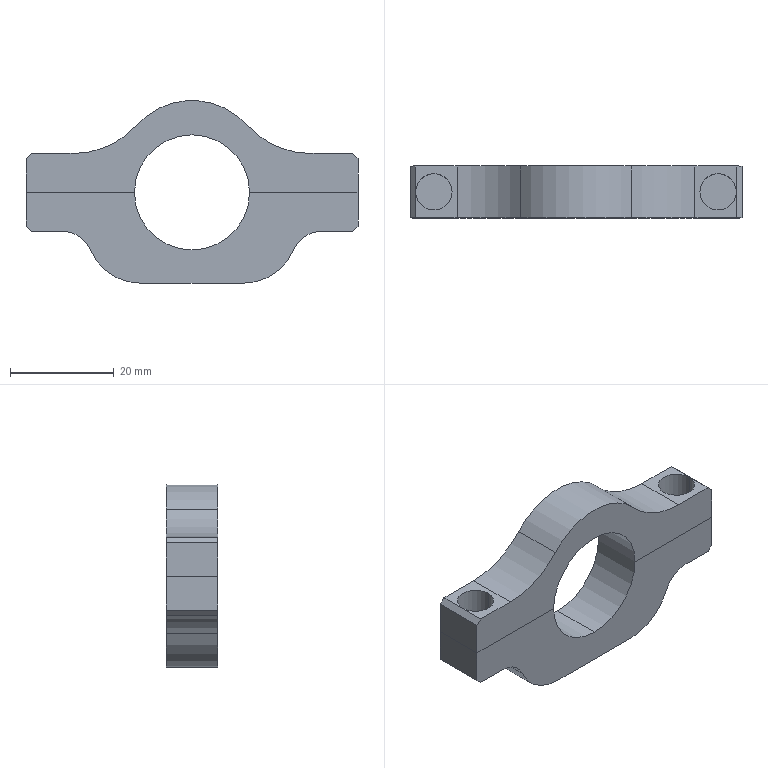Part | SolidWorks | features ICE 2, Chamfer 1, Extrusion 1, PLine 1 | 1 solid | 32 faces | box 64 x 10 x 35.214 mm | volume 11091 mm3 | plane 19 | cylinder 13 | commonest cylinder face diameters 7 x4 11.692 x2 21.037 x2 22.2 x2 33.122 x2 28.569 x1
STEP:
#1=CARTESIAN_POINT('',(0.,0.,-6.346));
#2=VERTEX_POINT('',#1);
#3=CARTESIAN_POINT('',(-11.1,0.,4.754));
#4=VERTEX_POINT('',#3);
#5=CARTESIAN_POINT('',(0.,0.,4.754));
#6=DIRECTION('',(0.,1.,0.));
#7=DIRECTION('',(0.,0.,1.));
#8=AXIS2_PLACEMENT_3D('',#5,#6,#7);
#9=CIRCLE('',#8,11.1);
#10=EDGE_CURVE('',#2,#4,#9,.T.);
#11=ORIENTED_EDGE('',*,*,#10,.F.);
#12=CARTESIAN_POINT('',(0.,10.,-6.346));
#13=VERTEX_POINT('',#12);
#14=CARTESIAN_POINT('',(0.,-10.,-6.346));
#15=DIRECTION('',(0.,1.,0.));
#16=VECTOR('',#15,1000.);
#17=LINE('',#14,#16);
#18=EDGE_CURVE('',#2,#13,#17,.T.);
#19=ORIENTED_EDGE('',*,*,#18,.T.);
#20=CARTESIAN_POINT('',(-11.1,10.,4.754));
#21=VERTEX_POINT('',#20);
#22=CARTESIAN_POINT('',(0.,10.,4.754));
#23=DIRECTION('',(0.,1.,0.));
#24=DIRECTION('',(0.,0.,1.));
#25=AXIS2_PLACEMENT_3D('',#22,#23,#24);
#26=CIRCLE('',#25,11.1);
#27=EDGE_CURVE('',#13,#21,#26,.T.);
#28=ORIENTED_EDGE('',*,*,#27,.T.);
#29=CARTESIAN_POINT('',(0.,10.,15.854));
#30=VERTEX_POINT('',#29);
#31=CARTESIAN_POINT('',(0.,10.,4.754));
#32=DIRECTION('',(0.,1.,0.));
#33=DIRECTION('',(0.,0.,1.));
#34=AXIS2_PLACEMENT_3D('',#31,#32,#33);
#35=CIRCLE('',#34,11.1);
#36=EDGE_CURVE('',#21,#30,#35,.T.);
#37=ORIENTED_EDGE('',*,*,#36,.T.);
#38=CARTESIAN_POINT('',(0.,0.,15.854));
#39=VERTEX_POINT('',#38);
#40=CARTESIAN_POINT('',(0.,-10.,15.854));
#41=DIRECTION('',(0.,1.,0.));
#42=VECTOR('',#41,1000.);
#43=LINE('',#40,#42);
#44=EDGE_CURVE('',#39,#30,#43,.T.);
#45=ORIENTED_EDGE('',*,*,#44,.F.);
#46=CARTESIAN_POINT('',(0.,0.,4.754));
#47=DIRECTION('',(0.,1.,0.));
#48=DIRECTION('',(0.,0.,1.));
#49=AXIS2_PLACEMENT_3D('',#46,#47,#48);
#50=CIRCLE('',#49,11.1);
#51=EDGE_CURVE('',#4,#39,#50,.T.);
#52=ORIENTED_EDGE('',*,*,#51,.F.);
#53=EDGE_LOOP('',(#11,#19,#28,#37,#45,#52));
#54=FACE_OUTER_BOUND('',#53,.T.);
#55=CARTESIAN_POINT('',(0.,-10.,4.754));
#56=DIRECTION('',(0.,1.,0.));
#57=DIRECTION('',(0.,0.,1.));
#58=AXIS2_PLACEMENT_3D('',#55,#56,#57);
#59=CYLINDRICAL_SURFACE('',#58,11.1);
#60=ADVANCED_FACE('',(#54),#59,.F.);
#61=CARTESIAN_POINT('',(-30.901,5.,12.254));
#62=VERTEX_POINT('',#61);
#63=CARTESIAN_POINT('',(-23.901,5.,12.254));
#64=VERTEX_POINT('',#63);
#65=CARTESIAN_POINT('',(-27.401,5.,12.254));
#66=DIRECTION('',(0.,0.,1.));
#67=DIRECTION('',(-1.,0.,0.));
#68=AXIS2_PLACEMENT_3D('',#65,#66,#67);
#69=CIRCLE('',#68,3.5);
#70=EDGE_CURVE('',#62,#64,#69,.T.);
#71=ORIENTED_EDGE('',*,*,#70,.T.);
#72=CARTESIAN_POINT('',(-23.901,5.,4.754));
#73=VERTEX_POINT('',#72);
#74=CARTESIAN_POINT('',(-23.901,5.,24.754));
#75=DIRECTION('',(0.,0.,-1.));
#76=VECTOR('',#75,1000.);
#77=LINE('',#74,#76);
#78=EDGE_CURVE('',#64,#73,#77,.T.);
#79=ORIENTED_EDGE('',*,*,#78,.T.);
#80=CARTESIAN_POINT('',(-30.901,5.,4.754));
#81=VERTEX_POINT('',#80);
#82=CARTESIAN_POINT('',(-27.401,5.,4.754));
#83=DIRECTION('',(0.,0.,1.));
#84=DIRECTION('',(-1.,0.,0.));
#85=AXIS2_PLACEMENT_3D('',#82,#83,#84);
#86=CIRCLE('',#85,3.5);
#87=EDGE_CURVE('',#81,#73,#86,.T.);
#88=ORIENTED_EDGE('',*,*,#87,.F.);
#89=CARTESIAN_POINT('',(-30.901,5.,24.754));
#90=DIRECTION('',(0.,0.,-1.));
#91=VECTOR('',#90,1000.);
#92=LINE('',#89,#91);
#93=EDGE_CURVE('',#62,#81,#92,.T.);
#94=ORIENTED_EDGE('',*,*,#93,.F.);
#95=EDGE_LOOP('',(#71,#79,#88,#94));
#96=FACE_OUTER_BOUND('',#95,.T.);
#97=CARTESIAN_POINT('',(-27.401,5.,24.754));
#98=DIRECTION('',(0.,0.,-1.));
#99=DIRECTION('',(-1.,0.,0.));
#100=AXIS2_PLACEMENT_3D('',#97,#98,#99);
#101=CYLINDRICAL_SURFACE('',#100,3.5);
#102=ADVANCED_FACE('',(#96),#101,.F.);
#103=CARTESIAN_POINT('',(30.901,5.,12.254));
#104=VERTEX_POINT('',#103);
#105=CARTESIAN_POINT('',(23.901,5.,12.254));
#106=VERTEX_POINT('',#105);
#107=CARTESIAN_POINT('',(27.401,5.,12.254));
#108=DIRECTION('',(0.,0.,-1.));
#109=DIRECTION('',(1.,0.,0.));
#110=AXIS2_PLACEMENT_3D('',#107,#108,#109);
#111=CIRCLE('',#110,3.5);
#112=EDGE_CURVE('',#104,#106,#111,.T.);
#113=ORIENTED_EDGE('',*,*,#112,.F.);
#114=CARTESIAN_POINT('',(30.901,5.,4.754));
#115=VERTEX_POINT('',#114);
#116=CARTESIAN_POINT('',(30.901,5.,24.754));
#117=DIRECTION('',(0.,0.,-1.));
#118=VECTOR('',#117,1000.);
#119=LINE('',#116,#118);
#120=EDGE_CURVE('',#104,#115,#119,.T.);
#121=ORIENTED_EDGE('',*,*,#120,.T.);
#122=CARTESIAN_POINT('',(23.901,5.,4.754));
#123=VERTEX_POINT('',#122);
#124=CARTESIAN_POINT('',(27.401,5.,4.754));
#125=DIRECTION('',(0.,0.,1.));
#126=DIRECTION('',(1.,0.,0.));
#127=AXIS2_PLACEMENT_3D('',#124,#125,#126);
#128=CIRCLE('',#127,3.5);
#129=EDGE_CURVE('',#123,#115,#128,.T.);
#130=ORIENTED_EDGE('',*,*,#129,.F.);
#131=CARTESIAN_POINT('',(23.901,5.,24.754));
#132=DIRECTION('',(0.,0.,-1.));
#133=VECTOR('',#132,1000.);
#134=LINE('',#131,#133);
#135=EDGE_CURVE('',#106,#123,#134,.T.);
#136=ORIENTED_EDGE('',*,*,#135,.F.);
#137=EDGE_LOOP('',(#113,#121,#130,#136));
#138=FACE_OUTER_BOUND('',#137,.T.);
#139=CARTESIAN_POINT('',(27.401,5.,24.754));
#140=DIRECTION('',(0.,0.,-1.));
#141=DIRECTION('',(-1.,0.,0.));
#142=AXIS2_PLACEMENT_3D('',#139,#140,#141);
#143=CYLINDRICAL_SURFACE('',#142,3.5);
#144=ADVANCED_FACE('',(#138),#143,.F.);
#145=CARTESIAN_POINT('',(-32.,0.,4.754));
#146=VERTEX_POINT('',#145);
#147=CARTESIAN_POINT('',(-32.,0.,11.254));
#148=VERTEX_POINT('',#147);
#149=CARTESIAN_POINT('',(-32.,0.,0.));
#150=DIRECTION('',(0.,0.,1.));
#151=VECTOR('',#150,1000.);
#152=LINE('',#149,#151);
#153=EDGE_CURVE('',#146,#148,#152,.T.);
#154=ORIENTED_EDGE('',*,*,#153,.T.);
#155=CARTESIAN_POINT('',(-32.,10.,11.254));
#156=VERTEX_POINT('',#155);
#157=CARTESIAN_POINT('',(-32.,10.,11.254));
#158=DIRECTION('',(0.,1.,0.));
#159=VECTOR('',#158,1000.);
#160=LINE('',#157,#159);
#161=EDGE_CURVE('',#148,#156,#160,.T.);
#162=ORIENTED_EDGE('',*,*,#161,.T.);
#163=CARTESIAN_POINT('',(-32.,10.,4.754));
#164=VERTEX_POINT('',#163);
#165=CARTESIAN_POINT('',(-32.,10.,0.));
#166=DIRECTION('',(0.,0.,1.));
#167=VECTOR('',#166,1000.);
#168=LINE('',#165,#167);
#169=EDGE_CURVE('',#164,#156,#168,.T.);
#170=ORIENTED_EDGE('',*,*,#169,.F.);
#171=CARTESIAN_POINT('',(-32.,10.,4.754));
#172=DIRECTION('',(0.,1.,0.));
#173=VECTOR('',#172,1000.);
#174=LINE('',#171,#173);
#175=EDGE_CURVE('',#146,#164,#174,.T.);
#176=ORIENTED_EDGE('',*,*,#175,.F.);
#177=EDGE_LOOP('',(#154,#162,#170,#176));
#178=FACE_OUTER_BOUND('',#177,.T.);
#179=CARTESIAN_POINT('',(-32.,10.,0.));
#180=DIRECTION('',(1.,0.,0.));
#181=DIRECTION('',(0.,0.,-1.));
#182=AXIS2_PLACEMENT_3D('',#179,#180,#181);
#183=PLANE('',#182);
#184=ADVANCED_FACE('',(#178),#183,.F.);
#185=CARTESIAN_POINT('',(32.,10.,4.754));
#186=VERTEX_POINT('',#185);
#187=CARTESIAN_POINT('',(32.,10.,11.254));
#188=VERTEX_POINT('',#187);
#189=CARTESIAN_POINT('',(32.,10.,0.));
#190=DIRECTION('',(0.,0.,1.));
#191=VECTOR('',#190,1000.);
#192=LINE('',#189,#191);
#193=EDGE_CURVE('',#186,#188,#192,.T.);
#194=ORIENTED_EDGE('',*,*,#193,.T.);
#195=CARTESIAN_POINT('',(32.,0.,11.254));
#196=VERTEX_POINT('',#195);
#197=CARTESIAN_POINT('',(32.,10.,11.254));
#198=DIRECTION('',(0.,-1.,0.));
#199=VECTOR('',#198,1000.);
#200=LINE('',#197,#199);
#201=EDGE_CURVE('',#188,#196,#200,.T.);
#202=ORIENTED_EDGE('',*,*,#201,.T.);
#203=CARTESIAN_POINT('',(32.,0.,4.754));
#204=VERTEX_POINT('',#203);
#205=CARTESIAN_POINT('',(32.,0.,0.));
#206=DIRECTION('',(0.,0.,1.));
#207=VECTOR('',#206,1000.);
#208=LINE('',#205,#207);
#209=EDGE_CURVE('',#204,#196,#208,.T.);
#210=ORIENTED_EDGE('',*,*,#209,.F.);
#211=CARTESIAN_POINT('',(32.,10.,4.754));
#212=DIRECTION('',(0.,1.,0.));
#213=VECTOR('',#212,1000.);
#214=LINE('',#211,#213);
#215=EDGE_CURVE('',#204,#186,#214,.T.);
#216=ORIENTED_EDGE('',*,*,#215,.T.);
#217=EDGE_LOOP('',(#194,#202,#210,#216));
#218=FACE_OUTER_BOUND('',#217,.T.);
#219=CARTESIAN_POINT('',(32.,10.,0.));
#220=DIRECTION('',(1.,0.,0.));
#221=DIRECTION('',(0.,0.,-1.));
#222=AXIS2_PLACEMENT_3D('',#219,#220,#221);
#223=PLANE('',#222);
#224=ADVANCED_FACE('',(#218),#223,.T.);
#225=ORIENTED_EDGE('',*,*,#36,.F.);
#226=CARTESIAN_POINT('',(0.,10.,4.754));
#227=DIRECTION('',(-1.,0.,0.));
#228=VECTOR('',#227,1000.);
#229=LINE('',#226,#228);
#230=EDGE_CURVE('',#21,#164,#229,.T.);
#231=ORIENTED_EDGE('',*,*,#230,.T.);
#232=ORIENTED_EDGE('',*,*,#169,.T.);
#233=CARTESIAN_POINT('',(-31.,10.,12.254));
#234=VERTEX_POINT('',#233);
#235=CARTESIAN_POINT('',(-21.627,10.,21.627));
#236=DIRECTION('',(0.7071,0.,0.7071));
#237=VECTOR('',#236,1000.);
#238=LINE('',#235,#237);
#239=EDGE_CURVE('',#156,#234,#238,.T.);
#240=ORIENTED_EDGE('',*,*,#239,.T.);
#241=CARTESIAN_POINT('',(-22.93,10.,12.254));
#242=VERTEX_POINT('',#241);
#243=CARTESIAN_POINT('',(0.,10.,12.254));
#244=DIRECTION('',(1.,0.,0.));
#245=VECTOR('',#244,1000.);
#246=LINE('',#243,#245);
#247=EDGE_CURVE('',#234,#242,#246,.T.);
#248=ORIENTED_EDGE('',*,*,#247,.T.);
#249=CARTESIAN_POINT('',(-10.619,10.,17.738));
#250=VERTEX_POINT('',#249);
#251=CARTESIAN_POINT('',(-22.93,10.,28.815));
#252=DIRECTION('',(0.,-1.,0.));
#253=DIRECTION('',(0.,0.,1.));
#254=AXIS2_PLACEMENT_3D('',#251,#252,#253);
#255=CIRCLE('',#254,16.561);
#256=EDGE_CURVE('',#242,#250,#255,.T.);
#257=ORIENTED_EDGE('',*,*,#256,.T.);
#258=CARTESIAN_POINT('',(10.619,10.,17.738));
#259=VERTEX_POINT('',#258);
#260=CARTESIAN_POINT('',(0.,10.,8.184));
#261=DIRECTION('',(0.,1.,0.));
#262=DIRECTION('',(0.,0.,1.));
#263=AXIS2_PLACEMENT_3D('',#260,#261,#262);
#264=CIRCLE('',#263,14.284);
#265=EDGE_CURVE('',#250,#259,#264,.T.);
#266=ORIENTED_EDGE('',*,*,#265,.T.);
#267=CARTESIAN_POINT('',(22.93,10.,12.254));
#268=VERTEX_POINT('',#267);
#269=CARTESIAN_POINT('',(22.93,10.,28.815));
#270=DIRECTION('',(0.,1.,0.));
#271=DIRECTION('',(0.,0.,1.));
#272=AXIS2_PLACEMENT_3D('',#269,#270,#271);
#273=CIRCLE('',#272,16.561);
#274=EDGE_CURVE('',#268,#259,#273,.T.);
#275=ORIENTED_EDGE('',*,*,#274,.F.);
#276=CARTESIAN_POINT('',(31.,10.,12.254));
#277=VERTEX_POINT('',#276);
#278=CARTESIAN_POINT('',(0.,10.,12.254));
#279=DIRECTION('',(-1.,0.,0.));
#280=VECTOR('',#279,1000.);
#281=LINE('',#278,#280);
#282=EDGE_CURVE('',#277,#268,#281,.T.);
#283=ORIENTED_EDGE('',*,*,#282,.F.);
#284=CARTESIAN_POINT('',(21.627,10.,21.627));
#285=DIRECTION('',(0.7071,0.,-0.7071));
#286=VECTOR('',#285,1000.);
#287=LINE('',#284,#286);
#288=EDGE_CURVE('',#277,#188,#287,.T.);
#289=ORIENTED_EDGE('',*,*,#288,.T.);
#290=ORIENTED_EDGE('',*,*,#193,.F.);
#291=CARTESIAN_POINT('',(11.1,10.,4.754));
#292=VERTEX_POINT('',#291);
#293=CARTESIAN_POINT('',(0.,10.,4.754));
#294=DIRECTION('',(-1.,0.,0.));
#295=VECTOR('',#294,1000.);
#296=LINE('',#293,#295);
#297=EDGE_CURVE('',#186,#292,#296,.T.);
#298=ORIENTED_EDGE('',*,*,#297,.T.);
#299=CARTESIAN_POINT('',(0.,10.,4.754));
#300=DIRECTION('',(0.,1.,0.));
#301=DIRECTION('',(0.,0.,1.));
#302=AXIS2_PLACEMENT_3D('',#299,#300,#301);
#303=CIRCLE('',#302,11.1);
#304=EDGE_CURVE('',#30,#292,#303,.T.);
#305=ORIENTED_EDGE('',*,*,#304,.F.);
#306=EDGE_LOOP('',(#225,#231,#232,#240,#248,#257,#266,#275,#283,#289,#290,#298,#305));
#307=FACE_OUTER_BOUND('',#306,.T.);
#308=CARTESIAN_POINT('',(0.,10.,0.));
#309=DIRECTION('',(0.,1.,0.));
#310=DIRECTION('',(0.,0.,1.));
#311=AXIS2_PLACEMENT_3D('',#308,#309,#310);
#312=PLANE('',#311);
#313=ADVANCED_FACE('',(#307),#312,.T.);
#314=CARTESIAN_POINT('',(0.,0.,4.754));
#315=DIRECTION('',(-1.,0.,0.));
#316=VECTOR('',#315,1000.);
#317=LINE('',#314,#316);
#318=EDGE_CURVE('',#4,#146,#317,.T.);
#319=ORIENTED_EDGE('',*,*,#318,.F.);
#320=ORIENTED_EDGE('',*,*,#51,.T.);
#321=CARTESIAN_POINT('',(11.1,0.,4.754));
#322=VERTEX_POINT('',#321);
#323=CARTESIAN_POINT('',(0.,0.,4.754));
#324=DIRECTION('',(0.,1.,0.));
#325=DIRECTION('',(0.,0.,1.));
#326=AXIS2_PLACEMENT_3D('',#323,#324,#325);
#327=CIRCLE('',#326,11.1);
#328=EDGE_CURVE('',#39,#322,#327,.T.);
#329=ORIENTED_EDGE('',*,*,#328,.T.);
#330=CARTESIAN_POINT('',(0.,0.,4.754));
#331=DIRECTION('',(-1.,0.,0.));
#332=VECTOR('',#331,1000.);
#333=LINE('',#330,#332);
#334=EDGE_CURVE('',#204,#322,#333,.T.);
#335=ORIENTED_EDGE('',*,*,#334,.F.);
#336=ORIENTED_EDGE('',*,*,#209,.T.);
#337=CARTESIAN_POINT('',(31.,0.,12.254));
#338=VERTEX_POINT('',#337);
#339=CARTESIAN_POINT('',(32.,0.,11.254));
#340=DIRECTION('',(-0.7071,0.,0.7071));
#341=VECTOR('',#340,1000.);
#342=LINE('',#339,#341);
#343=EDGE_CURVE('',#196,#338,#342,.T.);
#344=ORIENTED_EDGE('',*,*,#343,.T.);
#345=CARTESIAN_POINT('',(22.93,0.,12.254));
#346=VERTEX_POINT('',#345);
#347=CARTESIAN_POINT('',(0.,0.,12.254));
#348=DIRECTION('',(-1.,0.,0.));
#349=VECTOR('',#348,1000.);
#350=LINE('',#347,#349);
#351=EDGE_CURVE('',#338,#346,#350,.T.);
#352=ORIENTED_EDGE('',*,*,#351,.T.);
#353=CARTESIAN_POINT('',(10.619,0.,17.738));
#354=VERTEX_POINT('',#353);
#355=CARTESIAN_POINT('',(22.93,0.,28.815));
#356=DIRECTION('',(0.,1.,0.));
#357=DIRECTION('',(0.,0.,1.));
#358=AXIS2_PLACEMENT_3D('',#355,#356,#357);
#359=CIRCLE('',#358,16.561);
#360=EDGE_CURVE('',#346,#354,#359,.T.);
#361=ORIENTED_EDGE('',*,*,#360,.T.);
#362=CARTESIAN_POINT('',(-10.619,0.,17.738));
#363=VERTEX_POINT('',#362);
#364=CARTESIAN_POINT('',(0.,0.,8.184));
#365=DIRECTION('',(0.,1.,0.));
#366=DIRECTION('',(0.,0.,1.));
#367=AXIS2_PLACEMENT_3D('',#364,#365,#366);
#368=CIRCLE('',#367,14.284);
#369=EDGE_CURVE('',#363,#354,#368,.T.);
#370=ORIENTED_EDGE('',*,*,#369,.F.);
#371=CARTESIAN_POINT('',(-22.93,0.,12.254));
#372=VERTEX_POINT('',#371);
#373=CARTESIAN_POINT('',(-22.93,0.,28.815));
#374=DIRECTION('',(0.,-1.,0.));
#375=DIRECTION('',(0.,0.,1.));
#376=AXIS2_PLACEMENT_3D('',#373,#374,#375);
#377=CIRCLE('',#376,16.561);
#378=EDGE_CURVE('',#372,#363,#377,.T.);
#379=ORIENTED_EDGE('',*,*,#378,.F.);
#380=CARTESIAN_POINT('',(-31.,0.,12.254));
#381=VERTEX_POINT('',#380);
#382=CARTESIAN_POINT('',(0.,0.,12.254));
#383=DIRECTION('',(1.,0.,0.));
#384=VECTOR('',#383,1000.);
#385=LINE('',#382,#384);
#386=EDGE_CURVE('',#381,#372,#385,.T.);
#387=ORIENTED_EDGE('',*,*,#386,.F.);
#388=CARTESIAN_POINT('',(-31.,0.,12.254));
#389=DIRECTION('',(-0.7071,0.,-0.7071));
#390=VECTOR('',#389,1000.);
#391=LINE('',#388,#390);
#392=EDGE_CURVE('',#381,#148,#391,.T.);
#393=ORIENTED_EDGE('',*,*,#392,.T.);
#394=ORIENTED_EDGE('',*,*,#153,.F.);
#395=EDGE_LOOP('',(#319,#320,#329,#335,#336,#344,#352,#361,#370,#379,#387,#393,#394));
#396=FACE_OUTER_BOUND('',#395,.T.);
#397=CARTESIAN_POINT('',(0.,0.,0.));
#398=DIRECTION('',(0.,1.,0.));
#399=DIRECTION('',(0.,0.,1.));
#400=AXIS2_PLACEMENT_3D('',#397,#398,#399);
#401=PLANE('',#400);
#402=ADVANCED_FACE('',(#396),#401,.F.);
#403=CARTESIAN_POINT('',(9.924,0.,-12.746));
#404=VERTEX_POINT('',#403);
#405=CARTESIAN_POINT('',(19.614,0.,-6.318));
#406=VERTEX_POINT('',#405);
#407=CARTESIAN_POINT('',(9.924,0.,-2.227));
#408=DIRECTION('',(0.,-1.,0.));
#409=DIRECTION('',(0.,0.,1.));
#410=AXIS2_PLACEMENT_3D('',#407,#408,#409);
#411=CIRCLE('',#410,10.518);
#412=EDGE_CURVE('',#404,#406,#411,.T.);
#413=ORIENTED_EDGE('',*,*,#412,.F.);
#414=CARTESIAN_POINT('',(9.924,10.,-12.746));
#415=VERTEX_POINT('',#414);
#416=CARTESIAN_POINT('',(9.924,10.,-12.746));
#417=DIRECTION('',(0.,-1.,0.));
#418=VECTOR('',#417,1000.);
#419=LINE('',#416,#418);
#420=EDGE_CURVE('',#415,#404,#419,.T.);
#421=ORIENTED_EDGE('',*,*,#420,.F.);
#422=CARTESIAN_POINT('',(19.614,10.,-6.318));
#423=VERTEX_POINT('',#422);
#424=CARTESIAN_POINT('',(9.924,10.,-2.227));
#425=DIRECTION('',(0.,-1.,0.));
#426=DIRECTION('',(0.,0.,1.));
#427=AXIS2_PLACEMENT_3D('',#424,#425,#426);
#428=CIRCLE('',#427,10.518);
#429=EDGE_CURVE('',#415,#423,#428,.T.);
#430=ORIENTED_EDGE('',*,*,#429,.T.);
#431=CARTESIAN_POINT('',(19.614,10.,-6.318));
#432=DIRECTION('',(0.,-1.,0.));
#433=VECTOR('',#432,1000.);
#434=LINE('',#431,#433);
#435=EDGE_CURVE('',#423,#406,#434,.T.);
#436=ORIENTED_EDGE('',*,*,#435,.T.);
#437=EDGE_LOOP('',(#413,#421,#430,#436));
#438=FACE_OUTER_BOUND('',#437,.T.);
#439=CARTESIAN_POINT('',(9.924,10.,-2.227));
#440=DIRECTION('',(0.,-1.,0.));
#441=DIRECTION('',(0.,0.,-1.));
#442=AXIS2_PLACEMENT_3D('',#439,#440,#441);
#443=CYLINDRICAL_SURFACE('',#442,10.518);
#444=ADVANCED_FACE('',(#438),#443,.T.);
#445=CARTESIAN_POINT('',(-9.924,0.,-12.746));
#446=VERTEX_POINT('',#445);
#447=CARTESIAN_POINT('',(0.,0.,-12.746));
#448=DIRECTION('',(-1.,0.,0.));
#449=VECTOR('',#448,1000.);
#450=LINE('',#447,#449);
#451=EDGE_CURVE('',#404,#446,#450,.T.);
#452=ORIENTED_EDGE('',*,*,#451,.T.);
#453=CARTESIAN_POINT('',(-9.924,10.,-12.746));
#454=VERTEX_POINT('',#453);
#455=CARTESIAN_POINT('',(-9.924,10.,-12.746));
#456=DIRECTION('',(0.,-1.,0.));
#457=VECTOR('',#456,1000.);
#458=LINE('',#455,#457);
#459=EDGE_CURVE('',#454,#446,#458,.T.);
#460=ORIENTED_EDGE('',*,*,#459,.F.);
#461=CARTESIAN_POINT('',(0.,10.,-12.746));
#462=DIRECTION('',(-1.,0.,0.));
#463=VECTOR('',#462,1000.);
#464=LINE('',#461,#463);
#465=EDGE_CURVE('',#415,#454,#464,.T.);
#466=ORIENTED_EDGE('',*,*,#465,.F.);
#467=ORIENTED_EDGE('',*,*,#420,.T.);
#468=EDGE_LOOP('',(#452,#460,#466,#467));
#469=FACE_OUTER_BOUND('',#468,.T.);
#470=CARTESIAN_POINT('',(0.,10.,-12.746));
#471=DIRECTION('',(0.,0.,1.));
#472=DIRECTION('',(1.,0.,0.));
#473=AXIS2_PLACEMENT_3D('',#470,#471,#472);
#474=PLANE('',#473);
#475=ADVANCED_FACE('',(#469),#474,.F.);
#476=CARTESIAN_POINT('',(-19.614,0.,-6.318));
#477=VERTEX_POINT('',#476);
#478=CARTESIAN_POINT('',(-9.924,0.,-2.227));
#479=DIRECTION('',(0.,1.,0.));
#480=DIRECTION('',(0.,0.,1.));
#481=AXIS2_PLACEMENT_3D('',#478,#479,#480);
#482=CIRCLE('',#481,10.518);
#483=EDGE_CURVE('',#446,#477,#482,.T.);
#484=ORIENTED_EDGE('',*,*,#483,.T.);
#485=CARTESIAN_POINT('',(-19.614,10.,-6.318));
#486=VERTEX_POINT('',#485);
#487=CARTESIAN_POINT('',(-19.614,10.,-6.318));
#488=DIRECTION('',(0.,-1.,0.));
#489=VECTOR('',#488,1000.);
#490=LINE('',#487,#489);
#491=EDGE_CURVE('',#486,#477,#490,.T.);
#492=ORIENTED_EDGE('',*,*,#491,.F.);
#493=CARTESIAN_POINT('',(-9.924,10.,-2.227));
#494=DIRECTION('',(0.,1.,0.));
#495=DIRECTION('',(0.,0.,1.));
#496=AXIS2_PLACEMENT_3D('',#493,#494,#495);
#497=CIRCLE('',#496,10.518);
#498=EDGE_CURVE('',#454,#486,#497,.T.);
#499=ORIENTED_EDGE('',*,*,#498,.F.);
#500=ORIENTED_EDGE('',*,*,#459,.T.);
#501=EDGE_LOOP('',(#484,#492,#499,#500));
#502=FACE_OUTER_BOUND('',#501,.T.);
#503=CARTESIAN_POINT('',(-9.924,10.,-2.227));
#504=DIRECTION('',(0.,-1.,0.));
#505=DIRECTION('',(0.,0.,-1.));
#506=AXIS2_PLACEMENT_3D('',#503,#504,#505);
#507=CYLINDRICAL_SURFACE('',#506,10.518);
#508=ADVANCED_FACE('',(#502),#507,.T.);
#509=CARTESIAN_POINT('',(-25.,0.,-2.746));
#510=VERTEX_POINT('',#509);
#511=CARTESIAN_POINT('',(-25.,0.,-8.592));
#512=DIRECTION('',(0.,-1.,0.));
#513=DIRECTION('',(0.,0.,1.));
#514=AXIS2_PLACEMENT_3D('',#511,#512,#513);
#515=CIRCLE('',#514,5.846);
#516=EDGE_CURVE('',#477,#510,#515,.T.);
#517=ORIENTED_EDGE('',*,*,#516,.T.);
#518=CARTESIAN_POINT('',(-25.,10.,-2.746));
#519=VERTEX_POINT('',#518);
#520=CARTESIAN_POINT('',(-25.,10.,-2.746));
#521=DIRECTION('',(0.,-1.,0.));
#522=VECTOR('',#521,1000.);
#523=LINE('',#520,#522);
#524=EDGE_CURVE('',#519,#510,#523,.T.);
#525=ORIENTED_EDGE('',*,*,#524,.F.);
#526=CARTESIAN_POINT('',(-25.,10.,-8.592));
#527=DIRECTION('',(0.,-1.,0.));
#528=DIRECTION('',(0.,0.,1.));
#529=AXIS2_PLACEMENT_3D('',#526,#527,#528);
#530=CIRCLE('',#529,5.846);
#531=EDGE_CURVE('',#486,#519,#530,.T.);
#532=ORIENTED_EDGE('',*,*,#531,.F.);
#533=ORIENTED_EDGE('',*,*,#491,.T.);
#534=EDGE_LOOP('',(#517,#525,#532,#533));
#535=FACE_OUTER_BOUND('',#534,.T.);
#536=CARTESIAN_POINT('',(-25.,10.,-8.592));
#537=DIRECTION('',(0.,-1.,0.));
#538=DIRECTION('',(0.,0.,-1.));
#539=AXIS2_PLACEMENT_3D('',#536,#537,#538);
#540=CYLINDRICAL_SURFACE('',#539,5.846);
#541=ADVANCED_FACE('',(#535),#540,.F.);
#542=CARTESIAN_POINT('',(-31.,0.,-2.746));
#543=VERTEX_POINT('',#542);
#544=CARTESIAN_POINT('',(0.,0.,-2.746));
#545=DIRECTION('',(-1.,0.,0.));
#546=VECTOR('',#545,1000.);
#547=LINE('',#544,#546);
#548=EDGE_CURVE('',#510,#543,#547,.T.);
#549=ORIENTED_EDGE('',*,*,#548,.T.);
#550=CARTESIAN_POINT('',(-31.,10.,-2.746));
#551=VERTEX_POINT('',#550);
#552=CARTESIAN_POINT('',(-31.,10.,-2.746));
#553=DIRECTION('',(0.,1.,0.));
#554=VECTOR('',#553,1000.);
#555=LINE('',#552,#554);
#556=EDGE_CURVE('',#543,#551,#555,.T.);
#557=ORIENTED_EDGE('',*,*,#556,.T.);
#558=CARTESIAN_POINT('',(0.,10.,-2.746));
#559=DIRECTION('',(-1.,0.,0.));
#560=VECTOR('',#559,1000.);
#561=LINE('',#558,#560);
#562=EDGE_CURVE('',#519,#551,#561,.T.);
#563=ORIENTED_EDGE('',*,*,#562,.F.);
#564=ORIENTED_EDGE('',*,*,#524,.T.);
#565=EDGE_LOOP('',(#549,#557,#563,#564));
#566=FACE_OUTER_BOUND('',#565,.T.);
#567=CARTESIAN_POINT('',(0.,10.,-2.746));
#568=DIRECTION('',(0.,0.,1.));
#569=DIRECTION('',(1.,0.,0.));
#570=AXIS2_PLACEMENT_3D('',#567,#568,#569);
#571=PLANE('',#570);
#572=ADVANCED_FACE('',(#566),#571,.F.);
#573=CARTESIAN_POINT('',(-32.,10.,-1.746));
#574=VERTEX_POINT('',#573);
#575=CARTESIAN_POINT('',(-32.,10.,0.));
#576=DIRECTION('',(0.,0.,1.));
#577=VECTOR('',#576,1000.);
#578=LINE('',#575,#577);
#579=EDGE_CURVE('',#574,#164,#578,.T.);
#580=ORIENTED_EDGE('',*,*,#579,.F.);
#581=CARTESIAN_POINT('',(-32.,0.,-1.746));
#582=VERTEX_POINT('',#581);
#583=CARTESIAN_POINT('',(-32.,10.,-1.746));
#584=DIRECTION('',(0.,-1.,0.));
#585=VECTOR('',#584,1000.);
#586=LINE('',#583,#585);
#587=EDGE_CURVE('',#574,#582,#586,.T.);
#588=ORIENTED_EDGE('',*,*,#587,.T.);
#589=CARTESIAN_POINT('',(-32.,0.,0.));
#590=DIRECTION('',(0.,0.,1.));
#591=VECTOR('',#590,1000.);
#592=LINE('',#589,#591);
#593=EDGE_CURVE('',#582,#146,#592,.T.);
#594=ORIENTED_EDGE('',*,*,#593,.T.);
#595=ORIENTED_EDGE('',*,*,#175,.T.);
#596=EDGE_LOOP('',(#580,#588,#594,#595));
#597=FACE_OUTER_BOUND('',#596,.T.);
#598=CARTESIAN_POINT('',(-32.,10.,0.));
#599=DIRECTION('',(1.,0.,0.));
#600=DIRECTION('',(0.,0.,-1.));
#601=AXIS2_PLACEMENT_3D('',#598,#599,#600);
#602=PLANE('',#601);
#603=ADVANCED_FACE('',(#597),#602,.F.);
#604=ORIENTED_EDGE('',*,*,#70,.F.);
#605=CARTESIAN_POINT('',(-27.401,5.,12.254));
#606=DIRECTION('',(0.,0.,1.));
#607=DIRECTION('',(-1.,0.,0.));
#608=AXIS2_PLACEMENT_3D('',#605,#606,#607);
#609=CIRCLE('',#608,3.5);
#610=EDGE_CURVE('',#64,#62,#609,.T.);
#611=ORIENTED_EDGE('',*,*,#610,.F.);
#612=EDGE_LOOP('',(#604,#611));
#613=FACE_BOUND('',#612,.T.);
#614=ORIENTED_EDGE('',*,*,#247,.F.);
#615=CARTESIAN_POINT('',(-31.,10.,12.254));
#616=DIRECTION('',(0.,-1.,0.));
#617=VECTOR('',#616,1000.);
#618=LINE('',#615,#617);
#619=EDGE_CURVE('',#234,#381,#618,.T.);
#620=ORIENTED_EDGE('',*,*,#619,.T.);
#621=ORIENTED_EDGE('',*,*,#386,.T.);
#622=CARTESIAN_POINT('',(-22.93,10.,12.254));
#623=DIRECTION('',(0.,-1.,0.));
#624=VECTOR('',#623,1000.);
#625=LINE('',#622,#624);
#626=EDGE_CURVE('',#242,#372,#625,.T.);
#627=ORIENTED_EDGE('',*,*,#626,.F.);
#628=EDGE_LOOP('',(#614,#620,#621,#627));
#629=FACE_OUTER_BOUND('',#628,.T.);
#630=CARTESIAN_POINT('',(0.,10.,12.254));
#631=DIRECTION('',(0.,0.,-1.));
#632=DIRECTION('',(-1.,0.,0.));
#633=AXIS2_PLACEMENT_3D('',#630,#631,#632);
#634=PLANE('',#633);
#635=ADVANCED_FACE('',(#613,#629),#634,.F.);
#636=ORIENTED_EDGE('',*,*,#378,.T.);
#637=CARTESIAN_POINT('',(-10.619,10.,17.738));
#638=DIRECTION('',(0.,-1.,0.));
#639=VECTOR('',#638,1000.);
#640=LINE('',#637,#639);
#641=EDGE_CURVE('',#250,#363,#640,.T.);
#642=ORIENTED_EDGE('',*,*,#641,.F.);
#643=ORIENTED_EDGE('',*,*,#256,.F.);
#644=ORIENTED_EDGE('',*,*,#626,.T.);
#645=EDGE_LOOP('',(#636,#642,#643,#644));
#646=FACE_OUTER_BOUND('',#645,.T.);
#647=CARTESIAN_POINT('',(-22.93,10.,28.815));
#648=DIRECTION('',(0.,-1.,0.));
#649=DIRECTION('',(0.,0.,-1.));
#650=AXIS2_PLACEMENT_3D('',#647,#648,#649);
#651=CYLINDRICAL_SURFACE('',#650,16.561);
#652=ADVANCED_FACE('',(#646),#651,.F.);
#653=ORIENTED_EDGE('',*,*,#369,.T.);
#654=CARTESIAN_POINT('',(10.619,10.,17.738));
#655=DIRECTION('',(0.,-1.,0.));
#656=VECTOR('',#655,1000.);
#657=LINE('',#654,#656);
#658=EDGE_CURVE('',#259,#354,#657,.T.);
#659=ORIENTED_EDGE('',*,*,#658,.F.);
#660=ORIENTED_EDGE('',*,*,#265,.F.);
#661=ORIENTED_EDGE('',*,*,#641,.T.);
#662=EDGE_LOOP('',(#653,#659,#660,#661));
#663=FACE_OUTER_BOUND('',#662,.T.);
#664=CARTESIAN_POINT('',(0.,10.,8.184));
#665=DIRECTION('',(0.,-1.,0.));
#666=DIRECTION('',(0.,0.,-1.));
#667=AXIS2_PLACEMENT_3D('',#664,#665,#666);
#668=CYLINDRICAL_SURFACE('',#667,14.284);
#669=ADVANCED_FACE('',(#663),#668,.T.);
#670=ORIENTED_EDGE('',*,*,#360,.F.);
#671=CARTESIAN_POINT('',(22.93,10.,12.254));
#672=DIRECTION('',(0.,-1.,0.));
#673=VECTOR('',#672,1000.);
#674=LINE('',#671,#673);
#675=EDGE_CURVE('',#268,#346,#674,.T.);
#676=ORIENTED_EDGE('',*,*,#675,.F.);
#677=ORIENTED_EDGE('',*,*,#274,.T.);
#678=ORIENTED_EDGE('',*,*,#658,.T.);
#679=EDGE_LOOP('',(#670,#676,#677,#678));
#680=FACE_OUTER_BOUND('',#679,.T.);
#681=CARTESIAN_POINT('',(22.93,10.,28.815));
#682=DIRECTION('',(0.,-1.,0.));
#683=DIRECTION('',(0.,0.,-1.));
#684=AXIS2_PLACEMENT_3D('',#681,#682,#683);
#685=CYLINDRICAL_SURFACE('',#684,16.561);
#686=ADVANCED_FACE('',(#680),#685,.F.);
#687=CARTESIAN_POINT('',(27.401,5.,12.254));
#688=DIRECTION('',(0.,0.,-1.));
#689=DIRECTION('',(1.,0.,0.));
#690=AXIS2_PLACEMENT_3D('',#687,#688,#689);
#691=CIRCLE('',#690,3.5);
#692=EDGE_CURVE('',#106,#104,#691,.T.);
#693=ORIENTED_EDGE('',*,*,#692,.T.);
#694=ORIENTED_EDGE('',*,*,#112,.T.);
#695=EDGE_LOOP('',(#693,#694));
#696=FACE_BOUND('',#695,.T.);
#697=ORIENTED_EDGE('',*,*,#351,.F.);
#698=CARTESIAN_POINT('',(31.,10.,12.254));
#699=DIRECTION('',(0.,1.,0.));
#700=VECTOR('',#699,1000.);
#701=LINE('',#698,#700);
#702=EDGE_CURVE('',#338,#277,#701,.T.);
#703=ORIENTED_EDGE('',*,*,#702,.T.);
#704=ORIENTED_EDGE('',*,*,#282,.T.);
#705=ORIENTED_EDGE('',*,*,#675,.T.);
#706=EDGE_LOOP('',(#697,#703,#704,#705));
#707=FACE_OUTER_BOUND('',#706,.T.);
#708=CARTESIAN_POINT('',(0.,10.,12.254));
#709=DIRECTION('',(0.,0.,1.));
#710=DIRECTION('',(1.,0.,0.));
#711=AXIS2_PLACEMENT_3D('',#708,#709,#710);
#712=PLANE('',#711);
#713=ADVANCED_FACE('',(#696,#707),#712,.T.);
#714=CARTESIAN_POINT('',(32.,0.,-1.746));
#715=VERTEX_POINT('',#714);
#716=CARTESIAN_POINT('',(32.,0.,0.));
#717=DIRECTION('',(0.,0.,1.));
#718=VECTOR('',#717,1000.);
#719=LINE('',#716,#718);
#720=EDGE_CURVE('',#715,#204,#719,.T.);
#721=ORIENTED_EDGE('',*,*,#720,.F.);
#722=CARTESIAN_POINT('',(32.,10.,-1.746));
#723=VERTEX_POINT('',#722);
#724=CARTESIAN_POINT('',(32.,10.,-1.746));
#725=DIRECTION('',(0.,1.,0.));
#726=VECTOR('',#725,1000.);
#727=LINE('',#724,#726);
#728=EDGE_CURVE('',#715,#723,#727,.T.);
#729=ORIENTED_EDGE('',*,*,#728,.T.);
#730=CARTESIAN_POINT('',(32.,10.,0.));
#731=DIRECTION('',(0.,0.,1.));
#732=VECTOR('',#731,1000.);
#733=LINE('',#730,#732);
#734=EDGE_CURVE('',#723,#186,#733,.T.);
#735=ORIENTED_EDGE('',*,*,#734,.T.);
#736=ORIENTED_EDGE('',*,*,#215,.F.);
#737=EDGE_LOOP('',(#721,#729,#735,#736));
#738=FACE_OUTER_BOUND('',#737,.T.);
#739=CARTESIAN_POINT('',(32.,10.,0.));
#740=DIRECTION('',(1.,0.,0.));
#741=DIRECTION('',(0.,0.,-1.));
#742=AXIS2_PLACEMENT_3D('',#739,#740,#741);
#743=PLANE('',#742);
#744=ADVANCED_FACE('',(#738),#743,.T.);
#745=CARTESIAN_POINT('',(25.,10.,-2.746));
#746=VERTEX_POINT('',#745);
#747=CARTESIAN_POINT('',(31.,10.,-2.746));
#748=VERTEX_POINT('',#747);
#749=CARTESIAN_POINT('',(0.,10.,-2.746));
#750=DIRECTION('',(1.,0.,0.));
#751=VECTOR('',#750,1000.);
#752=LINE('',#749,#751);
#753=EDGE_CURVE('',#746,#748,#752,.T.);
#754=ORIENTED_EDGE('',*,*,#753,.T.);
#755=CARTESIAN_POINT('',(31.,0.,-2.746));
#756=VERTEX_POINT('',#755);
#757=CARTESIAN_POINT('',(31.,10.,-2.746));
#758=DIRECTION('',(0.,-1.,0.));
#759=VECTOR('',#758,1000.);
#760=LINE('',#757,#759);
#761=EDGE_CURVE('',#748,#756,#760,.T.);
#762=ORIENTED_EDGE('',*,*,#761,.T.);
#763=CARTESIAN_POINT('',(25.,0.,-2.746));
#764=VERTEX_POINT('',#763);
#765=CARTESIAN_POINT('',(0.,0.,-2.746));
#766=DIRECTION('',(1.,0.,0.));
#767=VECTOR('',#766,1000.);
#768=LINE('',#765,#767);
#769=EDGE_CURVE('',#764,#756,#768,.T.);
#770=ORIENTED_EDGE('',*,*,#769,.F.);
#771=CARTESIAN_POINT('',(25.,10.,-2.746));
#772=DIRECTION('',(0.,-1.,0.));
#773=VECTOR('',#772,1000.);
#774=LINE('',#771,#773);
#775=EDGE_CURVE('',#746,#764,#774,.T.);
#776=ORIENTED_EDGE('',*,*,#775,.F.);
#777=EDGE_LOOP('',(#754,#762,#770,#776));
#778=FACE_OUTER_BOUND('',#777,.T.);
#779=CARTESIAN_POINT('',(0.,10.,-2.746));
#780=DIRECTION('',(0.,0.,-1.));
#781=DIRECTION('',(-1.,0.,0.));
#782=AXIS2_PLACEMENT_3D('',#779,#780,#781);
#783=PLANE('',#782);
#784=ADVANCED_FACE('',(#778),#783,.T.);
#785=CARTESIAN_POINT('',(25.,0.,-8.592));
#786=DIRECTION('',(0.,1.,0.));
#787=DIRECTION('',(0.,0.,1.));
#788=AXIS2_PLACEMENT_3D('',#785,#786,#787);
#789=CIRCLE('',#788,5.846);
#790=EDGE_CURVE('',#406,#764,#789,.T.);
#791=ORIENTED_EDGE('',*,*,#790,.F.);
#792=ORIENTED_EDGE('',*,*,#435,.F.);
#793=CARTESIAN_POINT('',(25.,10.,-8.592));
#794=DIRECTION('',(0.,1.,0.));
#795=DIRECTION('',(0.,0.,1.));
#796=AXIS2_PLACEMENT_3D('',#793,#794,#795);
#797=CIRCLE('',#796,5.846);
#798=EDGE_CURVE('',#423,#746,#797,.T.);
#799=ORIENTED_EDGE('',*,*,#798,.T.);
#800=ORIENTED_EDGE('',*,*,#775,.T.);
#801=EDGE_LOOP('',(#791,#792,#799,#800));
#802=FACE_OUTER_BOUND('',#801,.T.);
#803=CARTESIAN_POINT('',(25.,10.,-8.592));
#804=DIRECTION('',(0.,-1.,0.));
#805=DIRECTION('',(0.,0.,-1.));
#806=AXIS2_PLACEMENT_3D('',#803,#804,#805);
#807=CYLINDRICAL_SURFACE('',#806,5.846);
#808=ADVANCED_FACE('',(#802),#807,.F.);
#809=CARTESIAN_POINT('',(0.,10.,4.754));
#810=DIRECTION('',(0.,1.,0.));
#811=DIRECTION('',(0.,0.,1.));
#812=AXIS2_PLACEMENT_3D('',#809,#810,#811);
#813=CIRCLE('',#812,11.1);
#814=EDGE_CURVE('',#292,#13,#813,.T.);
#815=ORIENTED_EDGE('',*,*,#814,.F.);
#816=ORIENTED_EDGE('',*,*,#297,.F.);
#817=ORIENTED_EDGE('',*,*,#734,.F.);
#818=CARTESIAN_POINT('',(16.873,10.,-16.873));
#819=DIRECTION('',(-0.7071,0.,-0.7071));
#820=VECTOR('',#819,1000.);
#821=LINE('',#818,#820);
#822=EDGE_CURVE('',#723,#748,#821,.T.);
#823=ORIENTED_EDGE('',*,*,#822,.T.);
#824=ORIENTED_EDGE('',*,*,#753,.F.);
#825=ORIENTED_EDGE('',*,*,#798,.F.);
#826=ORIENTED_EDGE('',*,*,#429,.F.);
#827=ORIENTED_EDGE('',*,*,#465,.T.);
#828=ORIENTED_EDGE('',*,*,#498,.T.);
#829=ORIENTED_EDGE('',*,*,#531,.T.);
#830=ORIENTED_EDGE('',*,*,#562,.T.);
#831=CARTESIAN_POINT('',(-16.873,10.,-16.873));
#832=DIRECTION('',(-0.7071,0.,0.7071));
#833=VECTOR('',#832,1000.);
#834=LINE('',#831,#833);
#835=EDGE_CURVE('',#551,#574,#834,.T.);
#836=ORIENTED_EDGE('',*,*,#835,.T.);
#837=ORIENTED_EDGE('',*,*,#579,.T.);
#838=ORIENTED_EDGE('',*,*,#230,.F.);
#839=ORIENTED_EDGE('',*,*,#27,.F.);
#840=EDGE_LOOP('',(#815,#816,#817,#823,#824,#825,#826,#827,#828,#829,#830,#836,#837,#838,#839));
#841=FACE_OUTER_BOUND('',#840,.T.);
#842=CARTESIAN_POINT('',(0.,10.,0.));
#843=DIRECTION('',(0.,1.,0.));
#844=DIRECTION('',(0.,0.,1.));
#845=AXIS2_PLACEMENT_3D('',#842,#843,#844);
#846=PLANE('',#845);
#847=ADVANCED_FACE('',(#841),#846,.T.);
#848=ORIENTED_EDGE('',*,*,#334,.T.);
#849=CARTESIAN_POINT('',(0.,0.,4.754));
#850=DIRECTION('',(0.,1.,0.));
#851=DIRECTION('',(0.,0.,1.));
#852=AXIS2_PLACEMENT_3D('',#849,#850,#851);
#853=CIRCLE('',#852,11.1);
#854=EDGE_CURVE('',#322,#2,#853,.T.);
#855=ORIENTED_EDGE('',*,*,#854,.T.);
#856=ORIENTED_EDGE('',*,*,#10,.T.);
#857=ORIENTED_EDGE('',*,*,#318,.T.);
#858=ORIENTED_EDGE('',*,*,#593,.F.);
#859=CARTESIAN_POINT('',(-32.,0.,-1.746));
#860=DIRECTION('',(0.7071,0.,-0.7071));
#861=VECTOR('',#860,1000.);
#862=LINE('',#859,#861);
#863=EDGE_CURVE('',#582,#543,#862,.T.);
#864=ORIENTED_EDGE('',*,*,#863,.T.);
#865=ORIENTED_EDGE('',*,*,#548,.F.);
#866=ORIENTED_EDGE('',*,*,#516,.F.);
#867=ORIENTED_EDGE('',*,*,#483,.F.);
#868=ORIENTED_EDGE('',*,*,#451,.F.);
#869=ORIENTED_EDGE('',*,*,#412,.T.);
#870=ORIENTED_EDGE('',*,*,#790,.T.);
#871=ORIENTED_EDGE('',*,*,#769,.T.);
#872=CARTESIAN_POINT('',(31.,0.,-2.746));
#873=DIRECTION('',(0.7071,0.,0.7071));
#874=VECTOR('',#873,1000.);
#875=LINE('',#872,#874);
#876=EDGE_CURVE('',#756,#715,#875,.T.);
#877=ORIENTED_EDGE('',*,*,#876,.T.);
#878=ORIENTED_EDGE('',*,*,#720,.T.);
#879=EDGE_LOOP('',(#848,#855,#856,#857,#858,#864,#865,#866,#867,#868,#869,#870,#871,#877,#878));
#880=FACE_OUTER_BOUND('',#879,.T.);
#881=CARTESIAN_POINT('',(0.,0.,0.));
#882=DIRECTION('',(0.,1.,0.));
#883=DIRECTION('',(0.,0.,1.));
#884=AXIS2_PLACEMENT_3D('',#881,#882,#883);
#885=PLANE('',#884);
#886=ADVANCED_FACE('',(#880),#885,.F.);
#887=ORIENTED_EDGE('',*,*,#239,.F.);
#888=ORIENTED_EDGE('',*,*,#161,.F.);
#889=ORIENTED_EDGE('',*,*,#392,.F.);
#890=ORIENTED_EDGE('',*,*,#619,.F.);
#891=EDGE_LOOP('',(#887,#888,#889,#890));
#892=FACE_OUTER_BOUND('',#891,.T.);
#893=CARTESIAN_POINT('',(-31.,10.,12.254));
#894=DIRECTION('',(0.7071,0.,-0.7071));
#895=DIRECTION('',(0.,-1.,0.));
#896=AXIS2_PLACEMENT_3D('',#893,#894,#895);
#897=PLANE('',#896);
#898=ADVANCED_FACE('',(#892),#897,.F.);
#899=ORIENTED_EDGE('',*,*,#835,.F.);
#900=ORIENTED_EDGE('',*,*,#556,.F.);
#901=ORIENTED_EDGE('',*,*,#863,.F.);
#902=ORIENTED_EDGE('',*,*,#587,.F.);
#903=EDGE_LOOP('',(#899,#900,#901,#902));
#904=FACE_OUTER_BOUND('',#903,.T.);
#905=CARTESIAN_POINT('',(-32.,10.,-1.746));
#906=DIRECTION('',(0.7071,0.,0.7071));
#907=DIRECTION('',(0.,-1.,0.));
#908=AXIS2_PLACEMENT_3D('',#905,#906,#907);
#909=PLANE('',#908);
#910=ADVANCED_FACE('',(#904),#909,.F.);
#911=ORIENTED_EDGE('',*,*,#288,.F.);
#912=ORIENTED_EDGE('',*,*,#702,.F.);
#913=ORIENTED_EDGE('',*,*,#343,.F.);
#914=ORIENTED_EDGE('',*,*,#201,.F.);
#915=EDGE_LOOP('',(#911,#912,#913,#914));
#916=FACE_OUTER_BOUND('',#915,.T.);
#917=CARTESIAN_POINT('',(32.,10.,11.254));
#918=DIRECTION('',(-0.7071,0.,-0.7071));
#919=DIRECTION('',(0.,-1.,0.));
#920=AXIS2_PLACEMENT_3D('',#917,#918,#919);
#921=PLANE('',#920);
#922=ADVANCED_FACE('',(#916),#921,.F.);
#923=ORIENTED_EDGE('',*,*,#822,.F.);
#924=ORIENTED_EDGE('',*,*,#728,.F.);
#925=ORIENTED_EDGE('',*,*,#876,.F.);
#926=ORIENTED_EDGE('',*,*,#761,.F.);
#927=EDGE_LOOP('',(#923,#924,#925,#926));
#928=FACE_OUTER_BOUND('',#927,.T.);
#929=CARTESIAN_POINT('',(31.,10.,-2.746));
#930=DIRECTION('',(-0.7071,0.,0.7071));
#931=DIRECTION('',(0.,-1.,0.));
#932=AXIS2_PLACEMENT_3D('',#929,#930,#931);
#933=PLANE('',#932);
#934=ADVANCED_FACE('',(#928),#933,.F.);
#935=ORIENTED_EDGE('',*,*,#120,.F.);
#936=ORIENTED_EDGE('',*,*,#692,.F.);
#937=ORIENTED_EDGE('',*,*,#135,.T.);
#938=CARTESIAN_POINT('',(27.401,5.,4.754));
#939=DIRECTION('',(0.,0.,1.));
#940=DIRECTION('',(1.,0.,0.));
#941=AXIS2_PLACEMENT_3D('',#938,#939,#940);
#942=CIRCLE('',#941,3.5);
#943=EDGE_CURVE('',#115,#123,#942,.T.);
#944=ORIENTED_EDGE('',*,*,#943,.F.);
#945=EDGE_LOOP('',(#935,#936,#937,#944));
#946=FACE_OUTER_BOUND('',#945,.T.);
#947=CARTESIAN_POINT('',(27.401,5.,24.754));
#948=DIRECTION('',(0.,0.,-1.));
#949=DIRECTION('',(-1.,0.,0.));
#950=AXIS2_PLACEMENT_3D('',#947,#948,#949);
#951=CYLINDRICAL_SURFACE('',#950,3.5);
#952=ADVANCED_FACE('',(#946),#951,.F.);
#953=ORIENTED_EDGE('',*,*,#129,.T.);
#954=ORIENTED_EDGE('',*,*,#943,.T.);
#955=EDGE_LOOP('',(#953,#954));
#956=FACE_OUTER_BOUND('',#955,.T.);
#957=CARTESIAN_POINT('',(27.401,5.,4.754));
#958=DIRECTION('',(0.,0.,1.));
#959=DIRECTION('',(1.,0.,0.));
#960=AXIS2_PLACEMENT_3D('',#957,#958,#959);
#961=PLANE('',#960);
#962=ADVANCED_FACE('',(#956),#961,.T.);
#963=ORIENTED_EDGE('',*,*,#78,.F.);
#964=ORIENTED_EDGE('',*,*,#610,.T.);
#965=ORIENTED_EDGE('',*,*,#93,.T.);
#966=CARTESIAN_POINT('',(-27.401,5.,4.754));
#967=DIRECTION('',(0.,0.,1.));
#968=DIRECTION('',(-1.,0.,0.));
#969=AXIS2_PLACEMENT_3D('',#966,#967,#968);
#970=CIRCLE('',#969,3.5);
#971=EDGE_CURVE('',#73,#81,#970,.T.);
#972=ORIENTED_EDGE('',*,*,#971,.F.);
#973=EDGE_LOOP('',(#963,#964,#965,#972));
#974=FACE_OUTER_BOUND('',#973,.T.);
#975=CARTESIAN_POINT('',(-27.401,5.,24.754));
#976=DIRECTION('',(0.,0.,-1.));
#977=DIRECTION('',(-1.,0.,0.));
#978=AXIS2_PLACEMENT_3D('',#975,#976,#977);
#979=CYLINDRICAL_SURFACE('',#978,3.5);
#980=ADVANCED_FACE('',(#974),#979,.F.);
#981=ORIENTED_EDGE('',*,*,#87,.T.);
#982=ORIENTED_EDGE('',*,*,#971,.T.);
#983=EDGE_LOOP('',(#981,#982));
#984=FACE_OUTER_BOUND('',#983,.T.);
#985=CARTESIAN_POINT('',(-27.401,5.,4.754));
#986=DIRECTION('',(0.,0.,-1.));
#987=DIRECTION('',(-1.,0.,0.));
#988=AXIS2_PLACEMENT_3D('',#985,#986,#987);
#989=PLANE('',#988);
#990=ADVANCED_FACE('',(#984),#989,.F.);
#991=ORIENTED_EDGE('',*,*,#18,.F.);
#992=ORIENTED_EDGE('',*,*,#854,.F.);
#993=ORIENTED_EDGE('',*,*,#328,.F.);
#994=ORIENTED_EDGE('',*,*,#44,.T.);
#995=ORIENTED_EDGE('',*,*,#304,.T.);
#996=ORIENTED_EDGE('',*,*,#814,.T.);
#997=EDGE_LOOP('',(#991,#992,#993,#994,#995,#996));
#998=FACE_OUTER_BOUND('',#997,.T.);
#999=CARTESIAN_POINT('',(0.,-10.,4.754));
#1000=DIRECTION('',(0.,1.,0.));
#1001=DIRECTION('',(0.,0.,1.));
#1002=AXIS2_PLACEMENT_3D('',#999,#1000,#1001);
#1003=CYLINDRICAL_SURFACE('',#1002,11.1);
#1004=ADVANCED_FACE('',(#998),#1003,.F.);
#1005=CLOSED_SHELL('',(#60,#102,#144,#184,#224,#313,#402,#444,#475,#508,#541,#572,#603,#635,#652,#669,#686,#713,#744,#784,#808,#847,#886,#898,#910,#922,#934,#952,#962,#980,#990,#1004));
#1006=MANIFOLD_SOLID_BREP('',#1005);
#1007=CARTESIAN_POINT('',(0.,0.,0.));
#1008=DIRECTION('',(0.,0.,1.));
#1009=DIRECTION('',(1.,0.,0.));
#1010=AXIS2_PLACEMENT_3D('',#1007,#1008,#1009);
#1011=(LENGTH_UNIT()NAMED_UNIT(*)SI_UNIT(.MILLI.,.METRE.));
#1012=UNCERTAINTY_MEASURE_WITH_UNIT(LENGTH_MEASURE(0.00001),#1011,'','');
#1013=(NAMED_UNIT(*)PLANE_ANGLE_UNIT()SI_UNIT($,.RADIAN.));
#1014=(NAMED_UNIT(*)SI_UNIT($,.STERADIAN.)SOLID_ANGLE_UNIT());
#1015=(GEOMETRIC_REPRESENTATION_CONTEXT(3)GLOBAL_UNCERTAINTY_ASSIGNED_CONTEXT((#1012))GLOBAL_UNIT_ASSIGNED_CONTEXT((#1011,#1013,#1014))REPRESENTATION_CONTEXT('',''));
#1016=ADVANCED_BREP_SHAPE_REPRESENTATION('',(#1006,#1010),#1015);